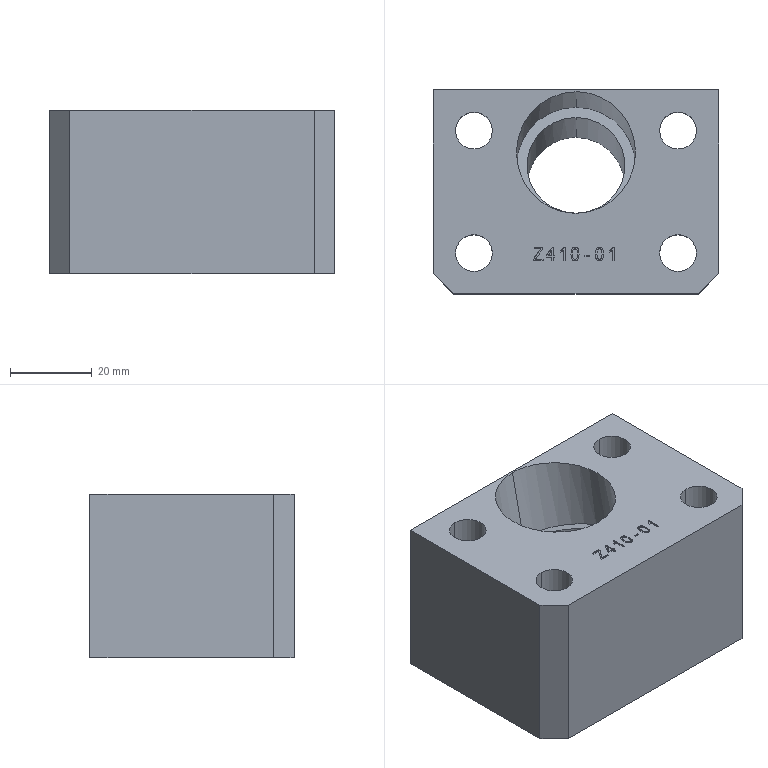Part | Creo | 1 solid | 131 faces | box 70 x 50 x 40 mm | volume 103877 mm3 | plane 57 | other 53 | cylinder 21 | commonest cylinder face diameters 9 x8 14 x8 24 x2 29.1 x2 45.582 x1